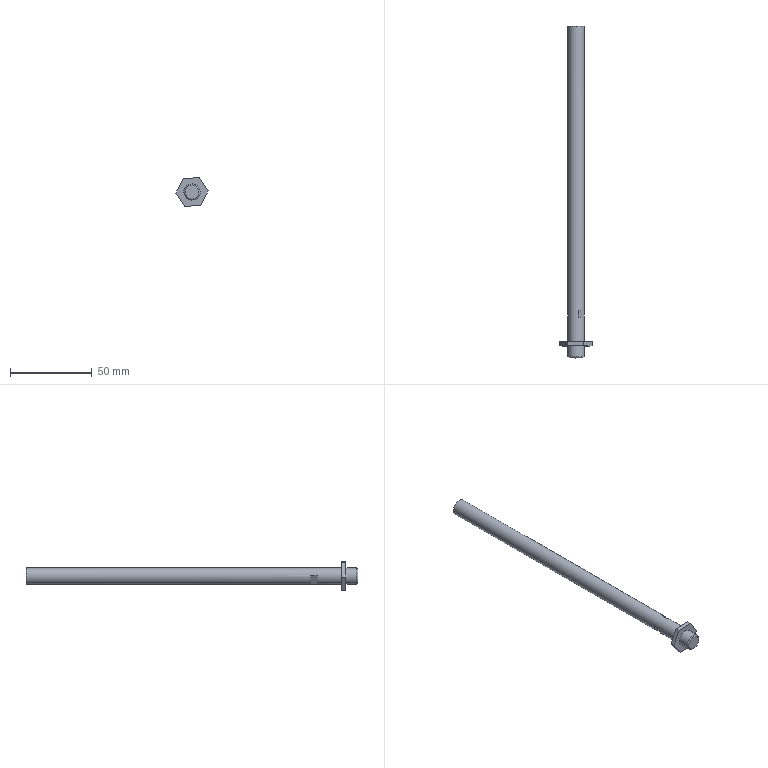Part | NX | features WGN01-25-100-Y-2-002 2 | 1 solid | 19 faces | box 19.589 x 203 x 17.595 mm | volume 16333 mm3 | plane 16 | cylinder 2 | cone 1 | commonest cylinder face diameters 10 x2
STEP:
#1=CARTESIAN_POINT('',(-1.665,234.332,130.166));
#2=VERTEX_POINT('',#1);
#3=CARTESIAN_POINT('',(-1.665,238.332,130.166));
#4=VERTEX_POINT('',#3);
#5=CARTESIAN_POINT('',(-1.665,238.332,130.166));
#6=DIRECTION('',(0.,-1.,0.));
#7=VECTOR('',#6,1000.);
#8=LINE('',#5,#7);
#9=EDGE_CURVE('',#2,#4,#8,.F.);
#10=ORIENTED_EDGE('',*,*,#9,.T.);
#11=CARTESIAN_POINT('',(-4.992,238.332,135.159));
#12=VERTEX_POINT('',#11);
#13=CARTESIAN_POINT('',(0.000006093,238.332,134.881));
#14=DIRECTION('',(0.,1.,0.));
#15=DIRECTION('',(-0.333,0.,-0.9429));
#16=AXIS2_PLACEMENT_3D('',#13,#14,#15);
#17=CIRCLE('',#16,5.);
#18=EDGE_CURVE('',#4,#12,#17,.T.);
#19=ORIENTED_EDGE('',*,*,#18,.T.);
#20=CARTESIAN_POINT('',(-4.992,234.332,135.159));
#21=VERTEX_POINT('',#20);
#22=CARTESIAN_POINT('',(-4.992,238.332,135.159));
#23=DIRECTION('',(0.,-1.,0.));
#24=VECTOR('',#23,1000.);
#25=LINE('',#22,#24);
#26=EDGE_CURVE('',#12,#21,#25,.T.);
#27=ORIENTED_EDGE('',*,*,#26,.T.);
#28=CARTESIAN_POINT('',(0.000006093,234.332,134.881));
#29=DIRECTION('',(0.,1.,0.));
#30=DIRECTION('',(-0.333,0.,-0.9429));
#31=AXIS2_PLACEMENT_3D('',#28,#29,#30);
#32=CIRCLE('',#31,5.);
#33=EDGE_CURVE('',#2,#21,#32,.T.);
#34=ORIENTED_EDGE('',*,*,#33,.F.);
#35=EDGE_LOOP('',(#10,#19,#27,#34));
#36=FACE_BOUND('',#35,.T.);
#37=CARTESIAN_POINT('',(0.000006093,219.166,139.881));
#38=VERTEX_POINT('',#37);
#39=CARTESIAN_POINT('',(0.000006093,219.166,134.881));
#40=DIRECTION('',(0.,1.,0.));
#41=DIRECTION('',(0.,0.,1.));
#42=AXIS2_PLACEMENT_3D('',#39,#40,#41);
#43=CIRCLE('',#42,5.);
#44=EDGE_CURVE('',#38,#38,#43,.T.);
#45=ORIENTED_EDGE('',*,*,#44,.T.);
#46=EDGE_LOOP('',(#45));
#47=FACE_BOUND('',#46,.T.);
#48=CARTESIAN_POINT('',(1.665,238.332,139.596));
#49=VERTEX_POINT('',#48);
#50=CARTESIAN_POINT('',(4.992,238.332,134.603));
#51=VERTEX_POINT('',#50);
#52=CARTESIAN_POINT('',(0.000006093,238.332,134.881));
#53=DIRECTION('',(0.,1.,0.));
#54=DIRECTION('',(0.333,0.,0.9429));
#55=AXIS2_PLACEMENT_3D('',#52,#53,#54);
#56=CIRCLE('',#55,5.);
#57=EDGE_CURVE('',#49,#51,#56,.T.);
#58=ORIENTED_EDGE('',*,*,#57,.T.);
#59=CARTESIAN_POINT('',(4.992,234.332,134.603));
#60=VERTEX_POINT('',#59);
#61=CARTESIAN_POINT('',(4.992,238.332,134.603));
#62=DIRECTION('',(0.,-1.,0.));
#63=VECTOR('',#62,1000.);
#64=LINE('',#61,#63);
#65=EDGE_CURVE('',#60,#51,#64,.F.);
#66=ORIENTED_EDGE('',*,*,#65,.F.);
#67=CARTESIAN_POINT('',(1.665,234.332,139.596));
#68=VERTEX_POINT('',#67);
#69=CARTESIAN_POINT('',(0.000006093,234.332,134.881));
#70=DIRECTION('',(0.,1.,0.));
#71=DIRECTION('',(0.333,0.,0.9429));
#72=AXIS2_PLACEMENT_3D('',#69,#70,#71);
#73=CIRCLE('',#72,5.);
#74=EDGE_CURVE('',#68,#60,#73,.T.);
#75=ORIENTED_EDGE('',*,*,#74,.F.);
#76=CARTESIAN_POINT('',(1.665,238.332,139.596));
#77=DIRECTION('',(0.,-1.,0.));
#78=VECTOR('',#77,1000.);
#79=LINE('',#76,#78);
#80=EDGE_CURVE('',#49,#68,#79,.T.);
#81=ORIENTED_EDGE('',*,*,#80,.F.);
#82=EDGE_LOOP('',(#58,#66,#75,#81));
#83=FACE_BOUND('',#82,.T.);
#84=CARTESIAN_POINT('',(-4.161,412.332,132.108));
#85=VERTEX_POINT('',#84);
#86=CARTESIAN_POINT('',(0.000006093,412.332,134.881));
#87=DIRECTION('',(0.,1.,0.));
#88=DIRECTION('',(-0.8321,0.,-0.5546));
#89=AXIS2_PLACEMENT_3D('',#86,#87,#88);
#90=CIRCLE('',#89,5.);
#91=EDGE_CURVE('',#85,#85,#90,.T.);
#92=ORIENTED_EDGE('',*,*,#91,.F.);
#93=EDGE_LOOP('',(#92));
#94=FACE_BOUND('',#93,.T.);
#95=CARTESIAN_POINT('',(0.000006093,412.332,134.881));
#96=DIRECTION('',(0.,1.,0.));
#97=DIRECTION('',(0.8321,0.,0.5546));
#98=AXIS2_PLACEMENT_3D('',#95,#96,#97);
#99=CYLINDRICAL_SURFACE('',#98,5.);
#100=ADVANCED_FACE('',(#36,#47,#83,#94),#99,.T.);
#101=CARTESIAN_POINT('',(-4.161,210.04,132.108));
#102=VERTEX_POINT('',#101);
#103=CARTESIAN_POINT('',(0.000006093,210.04,134.881));
#104=DIRECTION('',(0.,1.,0.));
#105=DIRECTION('',(-0.8321,0.,-0.5546));
#106=AXIS2_PLACEMENT_3D('',#103,#104,#105);
#107=CIRCLE('',#106,5.);
#108=EDGE_CURVE('',#102,#102,#107,.T.);
#109=ORIENTED_EDGE('',*,*,#108,.F.);
#110=EDGE_LOOP('',(#109));
#111=FACE_BOUND('',#110,.T.);
#112=CARTESIAN_POINT('',(-3.572,209.332,132.5));
#113=VERTEX_POINT('',#112);
#114=CARTESIAN_POINT('',(0.000006093,209.332,134.881));
#115=DIRECTION('',(0.,1.,0.));
#116=DIRECTION('',(-0.8321,0.,-0.5546));
#117=AXIS2_PLACEMENT_3D('',#114,#115,#116);
#118=CIRCLE('',#117,4.293);
#119=EDGE_CURVE('',#113,#113,#118,.T.);
#120=ORIENTED_EDGE('',*,*,#119,.T.);
#121=EDGE_LOOP('',(#120));
#122=FACE_BOUND('',#121,.T.);
#123=CARTESIAN_POINT('',(0.000006093,209.332,134.881));
#124=DIRECTION('',(0.,1.,0.));
#125=DIRECTION('',(0.8321,0.,0.5546));
#126=AXIS2_PLACEMENT_3D('',#123,#124,#125);
#127=CONICAL_SURFACE('',#126,4.293,0.7854);
#128=ADVANCED_FACE('',(#111,#122),#127,.T.);
#129=CARTESIAN_POINT('',(-4.161,216.666,132.108));
#130=VERTEX_POINT('',#129);
#131=CARTESIAN_POINT('',(0.000006093,216.666,134.881));
#132=DIRECTION('',(0.,1.,0.));
#133=DIRECTION('',(-0.8321,0.,-0.5546));
#134=AXIS2_PLACEMENT_3D('',#131,#132,#133);
#135=CIRCLE('',#134,5.);
#136=EDGE_CURVE('',#130,#130,#135,.T.);
#137=ORIENTED_EDGE('',*,*,#136,.F.);
#138=EDGE_LOOP('',(#137));
#139=FACE_BOUND('',#138,.T.);
#140=ORIENTED_EDGE('',*,*,#108,.T.);
#141=EDGE_LOOP('',(#140));
#142=FACE_BOUND('',#141,.T.);
#143=CARTESIAN_POINT('',(0.000006093,409.332,134.881));
#144=DIRECTION('',(0.,1.,0.));
#145=DIRECTION('',(0.8321,0.,0.5546));
#146=AXIS2_PLACEMENT_3D('',#143,#144,#145);
#147=CYLINDRICAL_SURFACE('',#146,5.);
#148=ADVANCED_FACE('',(#139,#142),#147,.T.);
#149=ORIENTED_EDGE('',*,*,#119,.F.);
#150=EDGE_LOOP('',(#149));
#151=FACE_BOUND('',#150,.T.);
#152=CARTESIAN_POINT('',(0.000006093,209.332,134.881));
#153=DIRECTION('',(0.,1.,0.));
#154=DIRECTION('',(0.8321,0.,0.5546));
#155=AXIS2_PLACEMENT_3D('',#152,#153,#154);
#156=PLANE('',#155);
#157=ADVANCED_FACE('',(#151),#156,.F.);
#158=CARTESIAN_POINT('',(4.351,216.666,143.679));
#159=VERTEX_POINT('',#158);
#160=CARTESIAN_POINT('',(9.795,216.666,135.512));
#161=VERTEX_POINT('',#160);
#162=CARTESIAN_POINT('',(4.351,216.666,143.679));
#163=DIRECTION('',(0.5546,0.,-0.8321));
#164=VECTOR('',#163,1000.);
#165=LINE('',#162,#164);
#166=EDGE_CURVE('',#159,#161,#165,.T.);
#167=ORIENTED_EDGE('',*,*,#166,.T.);
#168=CARTESIAN_POINT('',(9.795,219.166,135.512));
#169=VERTEX_POINT('',#168);
#170=CARTESIAN_POINT('',(9.795,222.666,135.512));
#171=DIRECTION('',(0.,-1.,0.));
#172=VECTOR('',#171,1000.);
#173=LINE('',#170,#172);
#174=EDGE_CURVE('',#169,#161,#173,.T.);
#175=ORIENTED_EDGE('',*,*,#174,.F.);
#176=CARTESIAN_POINT('',(4.351,219.166,143.679));
#177=VERTEX_POINT('',#176);
#178=CARTESIAN_POINT('',(4.351,219.166,143.679));
#179=DIRECTION('',(0.5546,0.,-0.8321));
#180=VECTOR('',#179,1000.);
#181=LINE('',#178,#180);
#182=EDGE_CURVE('',#177,#169,#181,.T.);
#183=ORIENTED_EDGE('',*,*,#182,.F.);
#184=CARTESIAN_POINT('',(4.351,222.666,143.679));
#185=DIRECTION('',(0.,-1.,0.));
#186=VECTOR('',#185,1000.);
#187=LINE('',#184,#186);
#188=EDGE_CURVE('',#177,#159,#187,.T.);
#189=ORIENTED_EDGE('',*,*,#188,.T.);
#190=EDGE_LOOP('',(#167,#175,#183,#189));
#191=FACE_BOUND('',#190,.T.);
#192=CARTESIAN_POINT('',(4.351,222.666,143.679));
#193=DIRECTION('',(-0.8321,0.,-0.5546));
#194=DIRECTION('',(0.,1.,0.));
#195=AXIS2_PLACEMENT_3D('',#192,#193,#194);
#196=PLANE('',#195);
#197=ADVANCED_FACE('',(#191),#196,.F.);
#198=CARTESIAN_POINT('',(5.443,216.666,126.714));
#199=VERTEX_POINT('',#198);
#200=CARTESIAN_POINT('',(9.795,216.666,135.512));
#201=DIRECTION('',(-0.4434,0.,-0.8963));
#202=VECTOR('',#201,1000.);
#203=LINE('',#200,#202);
#204=EDGE_CURVE('',#161,#199,#203,.T.);
#205=ORIENTED_EDGE('',*,*,#204,.T.);
#206=CARTESIAN_POINT('',(5.443,219.166,126.714));
#207=VERTEX_POINT('',#206);
#208=CARTESIAN_POINT('',(5.443,222.666,126.714));
#209=DIRECTION('',(0.,-1.,0.));
#210=VECTOR('',#209,1000.);
#211=LINE('',#208,#210);
#212=EDGE_CURVE('',#207,#199,#211,.T.);
#213=ORIENTED_EDGE('',*,*,#212,.F.);
#214=CARTESIAN_POINT('',(9.795,219.166,135.512));
#215=DIRECTION('',(-0.4434,0.,-0.8963));
#216=VECTOR('',#215,1000.);
#217=LINE('',#214,#216);
#218=EDGE_CURVE('',#169,#207,#217,.T.);
#219=ORIENTED_EDGE('',*,*,#218,.F.);
#220=ORIENTED_EDGE('',*,*,#174,.T.);
#221=EDGE_LOOP('',(#205,#213,#219,#220));
#222=FACE_BOUND('',#221,.T.);
#223=CARTESIAN_POINT('',(9.795,222.666,135.512));
#224=DIRECTION('',(-0.8963,0.,0.4434));
#225=DIRECTION('',(-0.4434,0.,-0.8963));
#226=AXIS2_PLACEMENT_3D('',#223,#224,#225);
#227=PLANE('',#226);
#228=ADVANCED_FACE('',(#222),#227,.F.);
#229=CARTESIAN_POINT('',(-4.351,216.666,126.084));
#230=VERTEX_POINT('',#229);
#231=CARTESIAN_POINT('',(5.443,216.666,126.714));
#232=DIRECTION('',(-0.9979,0.,-0.06422));
#233=VECTOR('',#232,1000.);
#234=LINE('',#231,#233);
#235=EDGE_CURVE('',#199,#230,#234,.T.);
#236=ORIENTED_EDGE('',*,*,#235,.T.);
#237=CARTESIAN_POINT('',(-4.351,219.166,126.084));
#238=VERTEX_POINT('',#237);
#239=CARTESIAN_POINT('',(-4.351,222.666,126.084));
#240=DIRECTION('',(0.,-1.,0.));
#241=VECTOR('',#240,1000.);
#242=LINE('',#239,#241);
#243=EDGE_CURVE('',#238,#230,#242,.T.);
#244=ORIENTED_EDGE('',*,*,#243,.F.);
#245=CARTESIAN_POINT('',(5.443,219.166,126.714));
#246=DIRECTION('',(-0.9979,0.,-0.06422));
#247=VECTOR('',#246,1000.);
#248=LINE('',#245,#247);
#249=EDGE_CURVE('',#207,#238,#248,.T.);
#250=ORIENTED_EDGE('',*,*,#249,.F.);
#251=ORIENTED_EDGE('',*,*,#212,.T.);
#252=EDGE_LOOP('',(#236,#244,#250,#251));
#253=FACE_BOUND('',#252,.T.);
#254=CARTESIAN_POINT('',(5.443,222.666,126.714));
#255=DIRECTION('',(-0.06422,0.,0.9979));
#256=DIRECTION('',(-0.9979,0.,-0.06422));
#257=AXIS2_PLACEMENT_3D('',#254,#255,#256);
#258=PLANE('',#257);
#259=ADVANCED_FACE('',(#253),#258,.F.);
#260=CARTESIAN_POINT('',(-9.795,216.666,134.251));
#261=VERTEX_POINT('',#260);
#262=CARTESIAN_POINT('',(-4.351,216.666,126.084));
#263=DIRECTION('',(-0.5546,0.,0.8321));
#264=VECTOR('',#263,1000.);
#265=LINE('',#262,#264);
#266=EDGE_CURVE('',#230,#261,#265,.T.);
#267=ORIENTED_EDGE('',*,*,#266,.T.);
#268=CARTESIAN_POINT('',(-9.795,219.166,134.251));
#269=VERTEX_POINT('',#268);
#270=CARTESIAN_POINT('',(-9.795,222.666,134.251));
#271=DIRECTION('',(0.,-1.,0.));
#272=VECTOR('',#271,1000.);
#273=LINE('',#270,#272);
#274=EDGE_CURVE('',#269,#261,#273,.T.);
#275=ORIENTED_EDGE('',*,*,#274,.F.);
#276=CARTESIAN_POINT('',(-4.351,219.166,126.084));
#277=DIRECTION('',(-0.5546,0.,0.8321));
#278=VECTOR('',#277,1000.);
#279=LINE('',#276,#278);
#280=EDGE_CURVE('',#238,#269,#279,.T.);
#281=ORIENTED_EDGE('',*,*,#280,.F.);
#282=ORIENTED_EDGE('',*,*,#243,.T.);
#283=EDGE_LOOP('',(#267,#275,#281,#282));
#284=FACE_BOUND('',#283,.T.);
#285=CARTESIAN_POINT('',(-4.351,222.666,126.084));
#286=DIRECTION('',(0.8321,0.,0.5546));
#287=DIRECTION('',(0.,-1.,0.));
#288=AXIS2_PLACEMENT_3D('',#285,#286,#287);
#289=PLANE('',#288);
#290=ADVANCED_FACE('',(#284),#289,.F.);
#291=CARTESIAN_POINT('',(-5.443,216.666,143.048));
#292=VERTEX_POINT('',#291);
#293=CARTESIAN_POINT('',(-9.795,216.666,134.251));
#294=DIRECTION('',(0.4434,0.,0.8963));
#295=VECTOR('',#294,1000.);
#296=LINE('',#293,#295);
#297=EDGE_CURVE('',#261,#292,#296,.T.);
#298=ORIENTED_EDGE('',*,*,#297,.T.);
#299=CARTESIAN_POINT('',(-5.443,219.166,143.048));
#300=VERTEX_POINT('',#299);
#301=CARTESIAN_POINT('',(-5.443,222.666,143.048));
#302=DIRECTION('',(0.,-1.,0.));
#303=VECTOR('',#302,1000.);
#304=LINE('',#301,#303);
#305=EDGE_CURVE('',#300,#292,#304,.T.);
#306=ORIENTED_EDGE('',*,*,#305,.F.);
#307=CARTESIAN_POINT('',(-9.795,219.166,134.251));
#308=DIRECTION('',(0.4434,0.,0.8963));
#309=VECTOR('',#308,1000.);
#310=LINE('',#307,#309);
#311=EDGE_CURVE('',#269,#300,#310,.T.);
#312=ORIENTED_EDGE('',*,*,#311,.F.);
#313=ORIENTED_EDGE('',*,*,#274,.T.);
#314=EDGE_LOOP('',(#298,#306,#312,#313));
#315=FACE_BOUND('',#314,.T.);
#316=CARTESIAN_POINT('',(-9.795,222.666,134.251));
#317=DIRECTION('',(0.8963,0.,-0.4434));
#318=DIRECTION('',(0.4434,0.,0.8963));
#319=AXIS2_PLACEMENT_3D('',#316,#317,#318);
#320=PLANE('',#319);
#321=ADVANCED_FACE('',(#315),#320,.F.);
#322=CARTESIAN_POINT('',(-5.443,216.666,143.048));
#323=DIRECTION('',(0.9979,0.,0.06422));
#324=VECTOR('',#323,1000.);
#325=LINE('',#322,#324);
#326=EDGE_CURVE('',#292,#159,#325,.T.);
#327=ORIENTED_EDGE('',*,*,#326,.T.);
#328=ORIENTED_EDGE('',*,*,#188,.F.);
#329=CARTESIAN_POINT('',(-5.443,219.166,143.048));
#330=DIRECTION('',(0.9979,0.,0.06422));
#331=VECTOR('',#330,1000.);
#332=LINE('',#329,#331);
#333=EDGE_CURVE('',#300,#177,#332,.T.);
#334=ORIENTED_EDGE('',*,*,#333,.F.);
#335=ORIENTED_EDGE('',*,*,#305,.T.);
#336=EDGE_LOOP('',(#327,#328,#334,#335));
#337=FACE_BOUND('',#336,.T.);
#338=CARTESIAN_POINT('',(-5.443,222.666,143.048));
#339=DIRECTION('',(0.06422,0.,-0.9979));
#340=DIRECTION('',(0.9979,0.,0.06422));
#341=AXIS2_PLACEMENT_3D('',#338,#339,#340);
#342=PLANE('',#341);
#343=ADVANCED_FACE('',(#337),#342,.F.);
#344=ORIENTED_EDGE('',*,*,#44,.F.);
#345=EDGE_LOOP('',(#344));
#346=FACE_BOUND('',#345,.T.);
#347=ORIENTED_EDGE('',*,*,#182,.T.);
#348=ORIENTED_EDGE('',*,*,#218,.T.);
#349=ORIENTED_EDGE('',*,*,#249,.T.);
#350=ORIENTED_EDGE('',*,*,#280,.T.);
#351=ORIENTED_EDGE('',*,*,#311,.T.);
#352=ORIENTED_EDGE('',*,*,#333,.T.);
#353=EDGE_LOOP('',(#347,#348,#349,#350,#351,#352));
#354=FACE_BOUND('',#353,.T.);
#355=CARTESIAN_POINT('',(0.000006093,219.166,134.881));
#356=DIRECTION('',(0.,1.,0.));
#357=DIRECTION('',(0.8321,0.,0.5546));
#358=AXIS2_PLACEMENT_3D('',#355,#356,#357);
#359=PLANE('',#358);
#360=ADVANCED_FACE('',(#346,#354),#359,.T.);
#361=ORIENTED_EDGE('',*,*,#136,.T.);
#362=EDGE_LOOP('',(#361));
#363=FACE_BOUND('',#362,.T.);
#364=ORIENTED_EDGE('',*,*,#166,.F.);
#365=ORIENTED_EDGE('',*,*,#326,.F.);
#366=ORIENTED_EDGE('',*,*,#297,.F.);
#367=ORIENTED_EDGE('',*,*,#266,.F.);
#368=ORIENTED_EDGE('',*,*,#235,.F.);
#369=ORIENTED_EDGE('',*,*,#204,.F.);
#370=EDGE_LOOP('',(#364,#365,#366,#367,#368,#369));
#371=FACE_BOUND('',#370,.T.);
#372=CARTESIAN_POINT('',(0.000006093,216.666,134.881));
#373=DIRECTION('',(0.,1.,0.));
#374=DIRECTION('',(0.8321,0.,0.5546));
#375=AXIS2_PLACEMENT_3D('',#372,#373,#374);
#376=PLANE('',#375);
#377=ADVANCED_FACE('',(#363,#371),#376,.F.);
#378=ORIENTED_EDGE('',*,*,#91,.T.);
#379=EDGE_LOOP('',(#378));
#380=FACE_BOUND('',#379,.T.);
#381=CARTESIAN_POINT('',(-2.773,412.332,139.042));
#382=DIRECTION('',(0.,-1.,0.));
#383=DIRECTION('',(-0.8321,0.,-0.5546));
#384=AXIS2_PLACEMENT_3D('',#381,#382,#383);
#385=PLANE('',#384);
#386=ADVANCED_FACE('',(#380),#385,.F.);
#387=CARTESIAN_POINT('',(4.992,234.332,134.603));
#388=DIRECTION('',(-0.5546,0.,0.8321));
#389=VECTOR('',#388,1000.);
#390=LINE('',#387,#389);
#391=EDGE_CURVE('',#60,#68,#390,.T.);
#392=ORIENTED_EDGE('',*,*,#391,.F.);
#393=ORIENTED_EDGE('',*,*,#65,.T.);
#394=CARTESIAN_POINT('',(4.992,238.332,134.603));
#395=DIRECTION('',(-0.5546,0.,0.8321));
#396=VECTOR('',#395,1000.);
#397=LINE('',#394,#396);
#398=EDGE_CURVE('',#51,#49,#397,.T.);
#399=ORIENTED_EDGE('',*,*,#398,.T.);
#400=ORIENTED_EDGE('',*,*,#80,.T.);
#401=EDGE_LOOP('',(#392,#393,#399,#400));
#402=FACE_BOUND('',#401,.T.);
#403=CARTESIAN_POINT('',(4.992,238.332,134.603));
#404=DIRECTION('',(0.8321,0.,0.5546));
#405=DIRECTION('',(0.,-1.,0.));
#406=AXIS2_PLACEMENT_3D('',#403,#404,#405);
#407=PLANE('',#406);
#408=ADVANCED_FACE('',(#402),#407,.T.);
#409=ORIENTED_EDGE('',*,*,#398,.F.);
#410=ORIENTED_EDGE('',*,*,#57,.F.);
#411=EDGE_LOOP('',(#409,#410));
#412=FACE_BOUND('',#411,.T.);
#413=CARTESIAN_POINT('',(0.000006093,238.332,134.881));
#414=DIRECTION('',(0.,1.,0.));
#415=DIRECTION('',(0.8321,0.,0.5546));
#416=AXIS2_PLACEMENT_3D('',#413,#414,#415);
#417=PLANE('',#416);
#418=ADVANCED_FACE('',(#412),#417,.F.);
#419=ORIENTED_EDGE('',*,*,#391,.T.);
#420=ORIENTED_EDGE('',*,*,#74,.T.);
#421=EDGE_LOOP('',(#419,#420));
#422=FACE_BOUND('',#421,.T.);
#423=CARTESIAN_POINT('',(0.000006093,234.332,134.881));
#424=DIRECTION('',(0.,1.,0.));
#425=DIRECTION('',(0.8321,0.,0.5546));
#426=AXIS2_PLACEMENT_3D('',#423,#424,#425);
#427=PLANE('',#426);
#428=ADVANCED_FACE('',(#422),#427,.T.);
#429=CARTESIAN_POINT('',(-4.992,234.332,135.159));
#430=DIRECTION('',(0.5546,0.,-0.8321));
#431=VECTOR('',#430,1000.);
#432=LINE('',#429,#431);
#433=EDGE_CURVE('',#21,#2,#432,.T.);
#434=ORIENTED_EDGE('',*,*,#433,.F.);
#435=ORIENTED_EDGE('',*,*,#26,.F.);
#436=CARTESIAN_POINT('',(-4.992,238.332,135.159));
#437=DIRECTION('',(0.5546,0.,-0.8321));
#438=VECTOR('',#437,1000.);
#439=LINE('',#436,#438);
#440=EDGE_CURVE('',#12,#4,#439,.T.);
#441=ORIENTED_EDGE('',*,*,#440,.T.);
#442=ORIENTED_EDGE('',*,*,#9,.F.);
#443=EDGE_LOOP('',(#434,#435,#441,#442));
#444=FACE_BOUND('',#443,.T.);
#445=CARTESIAN_POINT('',(-4.992,238.332,135.159));
#446=DIRECTION('',(-0.8321,0.,-0.5546));
#447=DIRECTION('',(0.,1.,0.));
#448=AXIS2_PLACEMENT_3D('',#445,#446,#447);
#449=PLANE('',#448);
#450=ADVANCED_FACE('',(#444),#449,.T.);
#451=ORIENTED_EDGE('',*,*,#18,.F.);
#452=ORIENTED_EDGE('',*,*,#440,.F.);
#453=EDGE_LOOP('',(#451,#452));
#454=FACE_BOUND('',#453,.T.);
#455=CARTESIAN_POINT('',(0.000006093,238.332,134.881));
#456=DIRECTION('',(0.,1.,0.));
#457=DIRECTION('',(0.8321,0.,0.5546));
#458=AXIS2_PLACEMENT_3D('',#455,#456,#457);
#459=PLANE('',#458);
#460=ADVANCED_FACE('',(#454),#459,.F.);
#461=ORIENTED_EDGE('',*,*,#433,.T.);
#462=ORIENTED_EDGE('',*,*,#33,.T.);
#463=EDGE_LOOP('',(#461,#462));
#464=FACE_BOUND('',#463,.T.);
#465=CARTESIAN_POINT('',(0.000006093,234.332,134.881));
#466=DIRECTION('',(0.,1.,0.));
#467=DIRECTION('',(0.8321,0.,0.5546));
#468=AXIS2_PLACEMENT_3D('',#465,#466,#467);
#469=PLANE('',#468);
#470=ADVANCED_FACE('',(#464),#469,.T.);
#471=CLOSED_SHELL('',(#100,#128,#148,#157,#197,#228,#259,#290,#321,#343,#360,#377,#386,#408,#418,#428,#450,#460,#470));
#472=MANIFOLD_SOLID_BREP('',#471);
#473=(LENGTH_UNIT()NAMED_UNIT(*)SI_UNIT(.MILLI.,.METRE.));
#474=UNCERTAINTY_MEASURE_WITH_UNIT(LENGTH_MEASURE(0.00001),#473,'','');
#475=(NAMED_UNIT(*)PLANE_ANGLE_UNIT()SI_UNIT($,.RADIAN.));
#476=(NAMED_UNIT(*)SI_UNIT($,.STERADIAN.)SOLID_ANGLE_UNIT());
#477=(GEOMETRIC_REPRESENTATION_CONTEXT(3)GLOBAL_UNCERTAINTY_ASSIGNED_CONTEXT((#474))GLOBAL_UNIT_ASSIGNED_CONTEXT((#473,#475,#476))REPRESENTATION_CONTEXT('',''));
#478=ADVANCED_BREP_SHAPE_REPRESENTATION('',(#472),#477);